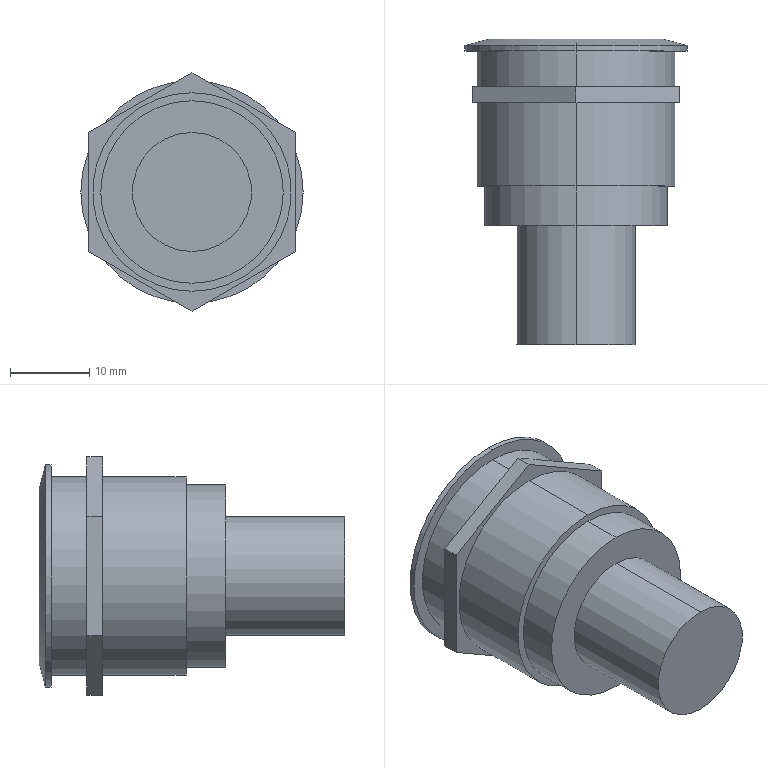Part | STEP file | MAIN_SWITCH_KNOB | 1 solid | 25 faces | box 28 x 38.5 x 30 mm | volume 14086 mm3 | plane 13 | cylinder 10 | cone 2 | commonest cylinder face diameters 25 x4 15 x2 23 x2 28 x2
STEP:
#1=CARTESIAN_POINT('',(0.,-8.,-12.5));
#2=VERTEX_POINT('',#1);
#3=CARTESIAN_POINT('',(0.,-8.,12.5));
#4=VERTEX_POINT('',#3);
#5=CARTESIAN_POINT('',(0.,-8.,0.));
#6=DIRECTION('',(0.,-1.,0.));
#7=DIRECTION('',(0.,0.,-1.));
#8=AXIS2_PLACEMENT_3D('',#5,#6,#7);
#9=CIRCLE('',#8,12.5);
#10=EDGE_CURVE('',#2,#4,#9,.T.);
#11=ORIENTED_EDGE('',*,*,#10,.T.);
#12=CARTESIAN_POINT('',(0.,-18.5,12.5));
#13=VERTEX_POINT('',#12);
#14=CARTESIAN_POINT('',(0.,1.925,12.5));
#15=DIRECTION('',(0.,-1.,0.));
#16=VECTOR('',#15,1000.);
#17=LINE('',#14,#16);
#18=EDGE_CURVE('',#4,#13,#17,.T.);
#19=ORIENTED_EDGE('',*,*,#18,.T.);
#20=CARTESIAN_POINT('',(0.,-18.5,-12.5));
#21=VERTEX_POINT('',#20);
#22=CARTESIAN_POINT('',(0.,-18.5,0.));
#23=DIRECTION('',(0.,1.,0.));
#24=DIRECTION('',(0.,0.,-1.));
#25=AXIS2_PLACEMENT_3D('',#22,#23,#24);
#26=CIRCLE('',#25,12.5);
#27=EDGE_CURVE('',#13,#21,#26,.T.);
#28=ORIENTED_EDGE('',*,*,#27,.T.);
#29=CARTESIAN_POINT('',(0.,1.925,-12.5));
#30=DIRECTION('',(0.,-1.,0.));
#31=VECTOR('',#30,1000.);
#32=LINE('',#29,#31);
#33=EDGE_CURVE('',#2,#21,#32,.T.);
#34=ORIENTED_EDGE('',*,*,#33,.F.);
#35=EDGE_LOOP('',(#11,#19,#28,#34));
#36=FACE_OUTER_BOUND('',#35,.T.);
#37=CARTESIAN_POINT('',(0.,1.925,0.));
#38=DIRECTION('',(0.,-1.,0.));
#39=DIRECTION('',(0.,0.,-1.));
#40=AXIS2_PLACEMENT_3D('',#37,#38,#39);
#41=CYLINDRICAL_SURFACE('',#40,12.5);
#42=ADVANCED_FACE('',(#36),#41,.T.);
#43=CARTESIAN_POINT('',(0.,-18.5,11.5));
#44=VERTEX_POINT('',#43);
#45=CARTESIAN_POINT('',(0.,-18.5,-11.5));
#46=VERTEX_POINT('',#45);
#47=CARTESIAN_POINT('',(0.,-18.5,0.));
#48=DIRECTION('',(0.,1.,0.));
#49=DIRECTION('',(0.,0.,-1.));
#50=AXIS2_PLACEMENT_3D('',#47,#48,#49);
#51=CIRCLE('',#50,11.5);
#52=EDGE_CURVE('',#44,#46,#51,.T.);
#53=ORIENTED_EDGE('',*,*,#52,.F.);
#54=CARTESIAN_POINT('',(0.,-23.5,11.5));
#55=VERTEX_POINT('',#54);
#56=CARTESIAN_POINT('',(0.,1.925,11.5));
#57=DIRECTION('',(0.,-1.,0.));
#58=VECTOR('',#57,1000.);
#59=LINE('',#56,#58);
#60=EDGE_CURVE('',#44,#55,#59,.T.);
#61=ORIENTED_EDGE('',*,*,#60,.T.);
#62=CARTESIAN_POINT('',(0.,-23.5,-11.5));
#63=VERTEX_POINT('',#62);
#64=CARTESIAN_POINT('',(0.,-23.5,0.));
#65=DIRECTION('',(0.,1.,0.));
#66=DIRECTION('',(0.,0.,-1.));
#67=AXIS2_PLACEMENT_3D('',#64,#65,#66);
#68=CIRCLE('',#67,11.5);
#69=EDGE_CURVE('',#55,#63,#68,.T.);
#70=ORIENTED_EDGE('',*,*,#69,.T.);
#71=CARTESIAN_POINT('',(0.,1.925,-11.5));
#72=DIRECTION('',(0.,-1.,0.));
#73=VECTOR('',#72,1000.);
#74=LINE('',#71,#73);
#75=EDGE_CURVE('',#46,#63,#74,.T.);
#76=ORIENTED_EDGE('',*,*,#75,.F.);
#77=EDGE_LOOP('',(#53,#61,#70,#76));
#78=FACE_OUTER_BOUND('',#77,.T.);
#79=CARTESIAN_POINT('',(0.,1.925,0.));
#80=DIRECTION('',(0.,-1.,0.));
#81=DIRECTION('',(0.,0.,-1.));
#82=AXIS2_PLACEMENT_3D('',#79,#80,#81);
#83=CYLINDRICAL_SURFACE('',#82,11.5);
#84=ADVANCED_FACE('',(#78),#83,.T.);
#85=CARTESIAN_POINT('',(0.,-23.5,7.5));
#86=VERTEX_POINT('',#85);
#87=CARTESIAN_POINT('',(0.,-23.5,-7.5));
#88=VERTEX_POINT('',#87);
#89=CARTESIAN_POINT('',(0.,-23.5,0.));
#90=DIRECTION('',(0.,1.,0.));
#91=DIRECTION('',(0.,0.,-1.));
#92=AXIS2_PLACEMENT_3D('',#89,#90,#91);
#93=CIRCLE('',#92,7.5);
#94=EDGE_CURVE('',#86,#88,#93,.T.);
#95=ORIENTED_EDGE('',*,*,#94,.F.);
#96=CARTESIAN_POINT('',(0.,-38.5,7.5));
#97=VERTEX_POINT('',#96);
#98=CARTESIAN_POINT('',(0.,1.925,7.5));
#99=DIRECTION('',(0.,-1.,0.));
#100=VECTOR('',#99,1000.);
#101=LINE('',#98,#100);
#102=EDGE_CURVE('',#86,#97,#101,.T.);
#103=ORIENTED_EDGE('',*,*,#102,.T.);
#104=CARTESIAN_POINT('',(0.,-38.5,-7.5));
#105=VERTEX_POINT('',#104);
#106=CARTESIAN_POINT('',(0.,-38.5,0.));
#107=DIRECTION('',(0.,1.,0.));
#108=DIRECTION('',(0.,0.,-1.));
#109=AXIS2_PLACEMENT_3D('',#106,#107,#108);
#110=CIRCLE('',#109,7.5);
#111=EDGE_CURVE('',#97,#105,#110,.T.);
#112=ORIENTED_EDGE('',*,*,#111,.T.);
#113=CARTESIAN_POINT('',(0.,1.925,-7.5));
#114=DIRECTION('',(0.,-1.,0.));
#115=VECTOR('',#114,1000.);
#116=LINE('',#113,#115);
#117=EDGE_CURVE('',#88,#105,#116,.T.);
#118=ORIENTED_EDGE('',*,*,#117,.F.);
#119=EDGE_LOOP('',(#95,#103,#112,#118));
#120=FACE_OUTER_BOUND('',#119,.T.);
#121=CARTESIAN_POINT('',(0.,1.925,0.));
#122=DIRECTION('',(0.,-1.,0.));
#123=DIRECTION('',(0.,0.,-1.));
#124=AXIS2_PLACEMENT_3D('',#121,#122,#123);
#125=CYLINDRICAL_SURFACE('',#124,7.5);
#126=ADVANCED_FACE('',(#120),#125,.T.);
#127=CARTESIAN_POINT('',(0.,-1.5,-12.5));
#128=VERTEX_POINT('',#127);
#129=CARTESIAN_POINT('',(0.,-1.5,12.5));
#130=VERTEX_POINT('',#129);
#131=CARTESIAN_POINT('',(0.,-1.5,0.));
#132=DIRECTION('',(0.,-1.,0.));
#133=DIRECTION('',(0.,0.,-1.));
#134=AXIS2_PLACEMENT_3D('',#131,#132,#133);
#135=CIRCLE('',#134,12.5);
#136=EDGE_CURVE('',#128,#130,#135,.T.);
#137=ORIENTED_EDGE('',*,*,#136,.T.);
#138=CARTESIAN_POINT('',(0.,-6.,12.5));
#139=VERTEX_POINT('',#138);
#140=CARTESIAN_POINT('',(0.,1.925,12.5));
#141=DIRECTION('',(0.,-1.,0.));
#142=VECTOR('',#141,1000.);
#143=LINE('',#140,#142);
#144=EDGE_CURVE('',#130,#139,#143,.T.);
#145=ORIENTED_EDGE('',*,*,#144,.T.);
#146=CARTESIAN_POINT('',(0.,-6.,-12.5));
#147=VERTEX_POINT('',#146);
#148=CARTESIAN_POINT('',(0.,-6.,0.));
#149=DIRECTION('',(0.,-1.,0.));
#150=DIRECTION('',(0.,0.,-1.));
#151=AXIS2_PLACEMENT_3D('',#148,#149,#150);
#152=CIRCLE('',#151,12.5);
#153=EDGE_CURVE('',#147,#139,#152,.T.);
#154=ORIENTED_EDGE('',*,*,#153,.F.);
#155=CARTESIAN_POINT('',(0.,1.925,-12.5));
#156=DIRECTION('',(0.,-1.,0.));
#157=VECTOR('',#156,1000.);
#158=LINE('',#155,#157);
#159=EDGE_CURVE('',#128,#147,#158,.T.);
#160=ORIENTED_EDGE('',*,*,#159,.F.);
#161=EDGE_LOOP('',(#137,#145,#154,#160));
#162=FACE_OUTER_BOUND('',#161,.T.);
#163=CARTESIAN_POINT('',(0.,1.925,0.));
#164=DIRECTION('',(0.,-1.,0.));
#165=DIRECTION('',(0.,0.,-1.));
#166=AXIS2_PLACEMENT_3D('',#163,#164,#165);
#167=CYLINDRICAL_SURFACE('',#166,12.5);
#168=ADVANCED_FACE('',(#162),#167,.T.);
#169=CARTESIAN_POINT('',(0.,-0.8,-14.));
#170=VERTEX_POINT('',#169);
#171=CARTESIAN_POINT('',(0.,-0.8,14.));
#172=VERTEX_POINT('',#171);
#173=CARTESIAN_POINT('',(0.,-0.8,0.));
#174=DIRECTION('',(0.,-1.,0.));
#175=DIRECTION('',(0.,0.,-1.));
#176=AXIS2_PLACEMENT_3D('',#173,#174,#175);
#177=CIRCLE('',#176,14.);
#178=EDGE_CURVE('',#170,#172,#177,.T.);
#179=ORIENTED_EDGE('',*,*,#178,.T.);
#180=CARTESIAN_POINT('',(0.,-1.5,14.));
#181=VERTEX_POINT('',#180);
#182=CARTESIAN_POINT('',(0.,1.925,14.));
#183=DIRECTION('',(0.,-1.,0.));
#184=VECTOR('',#183,1000.);
#185=LINE('',#182,#184);
#186=EDGE_CURVE('',#172,#181,#185,.T.);
#187=ORIENTED_EDGE('',*,*,#186,.T.);
#188=CARTESIAN_POINT('',(0.,-1.5,-14.));
#189=VERTEX_POINT('',#188);
#190=CARTESIAN_POINT('',(0.,-1.5,0.));
#191=DIRECTION('',(0.,-1.,0.));
#192=DIRECTION('',(0.,0.,-1.));
#193=AXIS2_PLACEMENT_3D('',#190,#191,#192);
#194=CIRCLE('',#193,14.);
#195=EDGE_CURVE('',#189,#181,#194,.T.);
#196=ORIENTED_EDGE('',*,*,#195,.F.);
#197=CARTESIAN_POINT('',(0.,1.925,-14.));
#198=DIRECTION('',(0.,-1.,0.));
#199=VECTOR('',#198,1000.);
#200=LINE('',#197,#199);
#201=EDGE_CURVE('',#170,#189,#200,.T.);
#202=ORIENTED_EDGE('',*,*,#201,.F.);
#203=EDGE_LOOP('',(#179,#187,#196,#202));
#204=FACE_OUTER_BOUND('',#203,.T.);
#205=CARTESIAN_POINT('',(0.,1.925,0.));
#206=DIRECTION('',(0.,-1.,0.));
#207=DIRECTION('',(0.,0.,-1.));
#208=AXIS2_PLACEMENT_3D('',#205,#206,#207);
#209=CYLINDRICAL_SURFACE('',#208,14.);
#210=ADVANCED_FACE('',(#204),#209,.T.);
#211=CARTESIAN_POINT('',(0.,0.,-11.014));
#212=VERTEX_POINT('',#211);
#213=CARTESIAN_POINT('',(0.,0.,11.014));
#214=VERTEX_POINT('',#213);
#215=CARTESIAN_POINT('',(0.,0.,0.));
#216=DIRECTION('',(0.,-1.,0.));
#217=DIRECTION('',(0.,0.,-1.));
#218=AXIS2_PLACEMENT_3D('',#215,#216,#217);
#219=CIRCLE('',#218,11.014);
#220=EDGE_CURVE('',#212,#214,#219,.T.);
#221=ORIENTED_EDGE('',*,*,#220,.T.);
#222=CARTESIAN_POINT('',(0.,-0.8,14.));
#223=DIRECTION('',(0.,-0.2588,0.9659));
#224=VECTOR('',#223,1000.);
#225=LINE('',#222,#224);
#226=EDGE_CURVE('',#214,#172,#225,.T.);
#227=ORIENTED_EDGE('',*,*,#226,.T.);
#228=ORIENTED_EDGE('',*,*,#178,.F.);
#229=CARTESIAN_POINT('',(0.,-0.8,-14.));
#230=DIRECTION('',(0.,-0.2588,-0.9659));
#231=VECTOR('',#230,1000.);
#232=LINE('',#229,#231);
#233=EDGE_CURVE('',#212,#170,#232,.T.);
#234=ORIENTED_EDGE('',*,*,#233,.F.);
#235=EDGE_LOOP('',(#221,#227,#228,#234));
#236=FACE_OUTER_BOUND('',#235,.T.);
#237=CARTESIAN_POINT('',(0.,-0.8,0.));
#238=DIRECTION('',(0.,-1.,0.));
#239=DIRECTION('',(0.,0.,-1.));
#240=AXIS2_PLACEMENT_3D('',#237,#238,#239);
#241=CONICAL_SURFACE('',#240,14.,1.309);
#242=ADVANCED_FACE('',(#236),#241,.T.);
#243=ORIENTED_EDGE('',*,*,#18,.F.);
#244=CARTESIAN_POINT('',(0.,-8.,0.));
#245=DIRECTION('',(0.,-1.,0.));
#246=DIRECTION('',(0.,0.,-1.));
#247=AXIS2_PLACEMENT_3D('',#244,#245,#246);
#248=CIRCLE('',#247,12.5);
#249=EDGE_CURVE('',#4,#2,#248,.T.);
#250=ORIENTED_EDGE('',*,*,#249,.T.);
#251=ORIENTED_EDGE('',*,*,#33,.T.);
#252=CARTESIAN_POINT('',(0.,-18.5,0.));
#253=DIRECTION('',(0.,1.,0.));
#254=DIRECTION('',(0.,0.,-1.));
#255=AXIS2_PLACEMENT_3D('',#252,#253,#254);
#256=CIRCLE('',#255,12.5);
#257=EDGE_CURVE('',#21,#13,#256,.T.);
#258=ORIENTED_EDGE('',*,*,#257,.T.);
#259=EDGE_LOOP('',(#243,#250,#251,#258));
#260=FACE_OUTER_BOUND('',#259,.T.);
#261=CARTESIAN_POINT('',(0.,1.925,0.));
#262=DIRECTION('',(0.,-1.,0.));
#263=DIRECTION('',(0.,0.,-1.));
#264=AXIS2_PLACEMENT_3D('',#261,#262,#263);
#265=CYLINDRICAL_SURFACE('',#264,12.5);
#266=ADVANCED_FACE('',(#260),#265,.T.);
#267=CARTESIAN_POINT('',(0.,-18.5,0.));
#268=DIRECTION('',(0.,1.,0.));
#269=DIRECTION('',(0.,0.,-1.));
#270=AXIS2_PLACEMENT_3D('',#267,#268,#269);
#271=CIRCLE('',#270,11.5);
#272=EDGE_CURVE('',#46,#44,#271,.T.);
#273=ORIENTED_EDGE('',*,*,#272,.T.);
#274=ORIENTED_EDGE('',*,*,#52,.T.);
#275=EDGE_LOOP('',(#273,#274));
#276=FACE_BOUND('',#275,.T.);
#277=ORIENTED_EDGE('',*,*,#257,.F.);
#278=ORIENTED_EDGE('',*,*,#27,.F.);
#279=EDGE_LOOP('',(#277,#278));
#280=FACE_OUTER_BOUND('',#279,.T.);
#281=CARTESIAN_POINT('',(0.,-18.5,0.));
#282=DIRECTION('',(0.,-1.,0.));
#283=DIRECTION('',(0.,0.,-1.));
#284=AXIS2_PLACEMENT_3D('',#281,#282,#283);
#285=PLANE('',#284);
#286=ADVANCED_FACE('',(#276,#280),#285,.T.);
#287=ORIENTED_EDGE('',*,*,#10,.F.);
#288=ORIENTED_EDGE('',*,*,#249,.F.);
#289=EDGE_LOOP('',(#287,#288));
#290=FACE_BOUND('',#289,.T.);
#291=CARTESIAN_POINT('',(0.,-8.,-15.));
#292=VERTEX_POINT('',#291);
#293=CARTESIAN_POINT('',(-12.99,-8.,-7.5));
#294=VERTEX_POINT('',#293);
#295=CARTESIAN_POINT('',(0.,-8.,-15.));
#296=DIRECTION('',(-0.866,0.,0.5));
#297=VECTOR('',#296,1000.);
#298=LINE('',#295,#297);
#299=EDGE_CURVE('',#292,#294,#298,.T.);
#300=ORIENTED_EDGE('',*,*,#299,.F.);
#301=CARTESIAN_POINT('',(12.99,-8.,-7.5));
#302=VERTEX_POINT('',#301);
#303=CARTESIAN_POINT('',(12.99,-8.,-7.5));
#304=DIRECTION('',(-0.866,0.,-0.5));
#305=VECTOR('',#304,1000.);
#306=LINE('',#303,#305);
#307=EDGE_CURVE('',#302,#292,#306,.T.);
#308=ORIENTED_EDGE('',*,*,#307,.F.);
#309=CARTESIAN_POINT('',(12.99,-8.,7.5));
#310=VERTEX_POINT('',#309);
#311=CARTESIAN_POINT('',(12.99,-8.,0.));
#312=DIRECTION('',(0.,0.,-1.));
#313=VECTOR('',#312,1000.);
#314=LINE('',#311,#313);
#315=EDGE_CURVE('',#310,#302,#314,.T.);
#316=ORIENTED_EDGE('',*,*,#315,.F.);
#317=CARTESIAN_POINT('',(0.,-8.,15.));
#318=VERTEX_POINT('',#317);
#319=CARTESIAN_POINT('',(0.,-8.,15.));
#320=DIRECTION('',(0.866,0.,-0.5));
#321=VECTOR('',#320,1000.);
#322=LINE('',#319,#321);
#323=EDGE_CURVE('',#318,#310,#322,.T.);
#324=ORIENTED_EDGE('',*,*,#323,.F.);
#325=CARTESIAN_POINT('',(-12.99,-8.,7.5));
#326=VERTEX_POINT('',#325);
#327=CARTESIAN_POINT('',(-12.99,-8.,7.5));
#328=DIRECTION('',(0.866,0.,0.5));
#329=VECTOR('',#328,1000.);
#330=LINE('',#327,#329);
#331=EDGE_CURVE('',#326,#318,#330,.T.);
#332=ORIENTED_EDGE('',*,*,#331,.F.);
#333=CARTESIAN_POINT('',(-12.99,-8.,0.));
#334=DIRECTION('',(0.,0.,1.));
#335=VECTOR('',#334,1000.);
#336=LINE('',#333,#335);
#337=EDGE_CURVE('',#294,#326,#336,.T.);
#338=ORIENTED_EDGE('',*,*,#337,.F.);
#339=EDGE_LOOP('',(#300,#308,#316,#324,#332,#338));
#340=FACE_OUTER_BOUND('',#339,.T.);
#341=CARTESIAN_POINT('',(0.,-8.,0.));
#342=DIRECTION('',(0.,1.,0.));
#343=DIRECTION('',(0.,0.,1.));
#344=AXIS2_PLACEMENT_3D('',#341,#342,#343);
#345=PLANE('',#344);
#346=ADVANCED_FACE('',(#290,#340),#345,.F.);
#347=ORIENTED_EDGE('',*,*,#60,.F.);
#348=ORIENTED_EDGE('',*,*,#272,.F.);
#349=ORIENTED_EDGE('',*,*,#75,.T.);
#350=CARTESIAN_POINT('',(0.,-23.5,0.));
#351=DIRECTION('',(0.,1.,0.));
#352=DIRECTION('',(0.,0.,-1.));
#353=AXIS2_PLACEMENT_3D('',#350,#351,#352);
#354=CIRCLE('',#353,11.5);
#355=EDGE_CURVE('',#63,#55,#354,.T.);
#356=ORIENTED_EDGE('',*,*,#355,.T.);
#357=EDGE_LOOP('',(#347,#348,#349,#356));
#358=FACE_OUTER_BOUND('',#357,.T.);
#359=CARTESIAN_POINT('',(0.,1.925,0.));
#360=DIRECTION('',(0.,-1.,0.));
#361=DIRECTION('',(0.,0.,-1.));
#362=AXIS2_PLACEMENT_3D('',#359,#360,#361);
#363=CYLINDRICAL_SURFACE('',#362,11.5);
#364=ADVANCED_FACE('',(#358),#363,.T.);
#365=CARTESIAN_POINT('',(-12.99,-6.,-7.5));
#366=VERTEX_POINT('',#365);
#367=CARTESIAN_POINT('',(-12.99,-8.,-7.5));
#368=DIRECTION('',(0.,-1.,0.));
#369=VECTOR('',#368,1000.);
#370=LINE('',#367,#369);
#371=EDGE_CURVE('',#366,#294,#370,.T.);
#372=ORIENTED_EDGE('',*,*,#371,.T.);
#373=ORIENTED_EDGE('',*,*,#337,.T.);
#374=CARTESIAN_POINT('',(-12.99,-6.,7.5));
#375=VERTEX_POINT('',#374);
#376=CARTESIAN_POINT('',(-12.99,-8.,7.5));
#377=DIRECTION('',(0.,1.,0.));
#378=VECTOR('',#377,1000.);
#379=LINE('',#376,#378);
#380=EDGE_CURVE('',#326,#375,#379,.T.);
#381=ORIENTED_EDGE('',*,*,#380,.T.);
#382=CARTESIAN_POINT('',(-12.99,-6.,-7.5));
#383=DIRECTION('',(0.,0.,-1.));
#384=VECTOR('',#383,1000.);
#385=LINE('',#382,#384);
#386=EDGE_CURVE('',#375,#366,#385,.T.);
#387=ORIENTED_EDGE('',*,*,#386,.T.);
#388=EDGE_LOOP('',(#372,#373,#381,#387));
#389=FACE_OUTER_BOUND('',#388,.T.);
#390=CARTESIAN_POINT('',(-12.99,-8.,-7.5));
#391=DIRECTION('',(-1.,0.,0.));
#392=DIRECTION('',(0.,0.,1.));
#393=AXIS2_PLACEMENT_3D('',#390,#391,#392);
#394=PLANE('',#393);
#395=ADVANCED_FACE('',(#389),#394,.T.);
#396=CARTESIAN_POINT('',(0.,-6.,-15.));
#397=VERTEX_POINT('',#396);
#398=CARTESIAN_POINT('',(0.,-8.,-15.));
#399=DIRECTION('',(0.,-1.,0.));
#400=VECTOR('',#399,1000.);
#401=LINE('',#398,#400);
#402=EDGE_CURVE('',#397,#292,#401,.T.);
#403=ORIENTED_EDGE('',*,*,#402,.T.);
#404=ORIENTED_EDGE('',*,*,#299,.T.);
#405=ORIENTED_EDGE('',*,*,#371,.F.);
#406=CARTESIAN_POINT('',(0.,-6.,-15.));
#407=DIRECTION('',(0.866,0.,-0.5));
#408=VECTOR('',#407,1000.);
#409=LINE('',#406,#408);
#410=EDGE_CURVE('',#366,#397,#409,.T.);
#411=ORIENTED_EDGE('',*,*,#410,.T.);
#412=EDGE_LOOP('',(#403,#404,#405,#411));
#413=FACE_OUTER_BOUND('',#412,.T.);
#414=CARTESIAN_POINT('',(0.,-8.,-15.));
#415=DIRECTION('',(-0.5,0.,-0.866));
#416=DIRECTION('',(-0.866,0.,0.5));
#417=AXIS2_PLACEMENT_3D('',#414,#415,#416);
#418=PLANE('',#417);
#419=ADVANCED_FACE('',(#413),#418,.T.);
#420=CARTESIAN_POINT('',(12.99,-6.,-7.5));
#421=VERTEX_POINT('',#420);
#422=CARTESIAN_POINT('',(12.99,-8.,-7.5));
#423=DIRECTION('',(0.,-1.,0.));
#424=VECTOR('',#423,1000.);
#425=LINE('',#422,#424);
#426=EDGE_CURVE('',#421,#302,#425,.T.);
#427=ORIENTED_EDGE('',*,*,#426,.T.);
#428=ORIENTED_EDGE('',*,*,#307,.T.);
#429=ORIENTED_EDGE('',*,*,#402,.F.);
#430=CARTESIAN_POINT('',(12.99,-6.,-7.5));
#431=DIRECTION('',(0.866,0.,0.5));
#432=VECTOR('',#431,1000.);
#433=LINE('',#430,#432);
#434=EDGE_CURVE('',#397,#421,#433,.T.);
#435=ORIENTED_EDGE('',*,*,#434,.T.);
#436=EDGE_LOOP('',(#427,#428,#429,#435));
#437=FACE_OUTER_BOUND('',#436,.T.);
#438=CARTESIAN_POINT('',(12.99,-8.,-7.5));
#439=DIRECTION('',(0.5,0.,-0.866));
#440=DIRECTION('',(-0.866,0.,-0.5));
#441=AXIS2_PLACEMENT_3D('',#438,#439,#440);
#442=PLANE('',#441);
#443=ADVANCED_FACE('',(#437),#442,.T.);
#444=CARTESIAN_POINT('',(12.99,-6.,7.5));
#445=VERTEX_POINT('',#444);
#446=CARTESIAN_POINT('',(12.99,-8.,7.5));
#447=DIRECTION('',(0.,-1.,0.));
#448=VECTOR('',#447,1000.);
#449=LINE('',#446,#448);
#450=EDGE_CURVE('',#445,#310,#449,.T.);
#451=ORIENTED_EDGE('',*,*,#450,.T.);
#452=ORIENTED_EDGE('',*,*,#315,.T.);
#453=ORIENTED_EDGE('',*,*,#426,.F.);
#454=CARTESIAN_POINT('',(12.99,-6.,7.5));
#455=DIRECTION('',(0.,0.,1.));
#456=VECTOR('',#455,1000.);
#457=LINE('',#454,#456);
#458=EDGE_CURVE('',#421,#445,#457,.T.);
#459=ORIENTED_EDGE('',*,*,#458,.T.);
#460=EDGE_LOOP('',(#451,#452,#453,#459));
#461=FACE_OUTER_BOUND('',#460,.T.);
#462=CARTESIAN_POINT('',(12.99,-8.,7.5));
#463=DIRECTION('',(1.,0.,0.));
#464=DIRECTION('',(0.,0.,-1.));
#465=AXIS2_PLACEMENT_3D('',#462,#463,#464);
#466=PLANE('',#465);
#467=ADVANCED_FACE('',(#461),#466,.T.);
#468=CARTESIAN_POINT('',(0.,-6.,15.));
#469=VERTEX_POINT('',#468);
#470=CARTESIAN_POINT('',(0.,-8.,15.));
#471=DIRECTION('',(0.,-1.,0.));
#472=VECTOR('',#471,1000.);
#473=LINE('',#470,#472);
#474=EDGE_CURVE('',#469,#318,#473,.T.);
#475=ORIENTED_EDGE('',*,*,#474,.T.);
#476=ORIENTED_EDGE('',*,*,#323,.T.);
#477=ORIENTED_EDGE('',*,*,#450,.F.);
#478=CARTESIAN_POINT('',(0.,-6.,15.));
#479=DIRECTION('',(-0.866,0.,0.5));
#480=VECTOR('',#479,1000.);
#481=LINE('',#478,#480);
#482=EDGE_CURVE('',#445,#469,#481,.T.);
#483=ORIENTED_EDGE('',*,*,#482,.T.);
#484=EDGE_LOOP('',(#475,#476,#477,#483));
#485=FACE_OUTER_BOUND('',#484,.T.);
#486=CARTESIAN_POINT('',(0.,-8.,15.));
#487=DIRECTION('',(0.5,0.,0.866));
#488=DIRECTION('',(0.866,0.,-0.5));
#489=AXIS2_PLACEMENT_3D('',#486,#487,#488);
#490=PLANE('',#489);
#491=ADVANCED_FACE('',(#485),#490,.T.);
#492=ORIENTED_EDGE('',*,*,#380,.F.);
#493=ORIENTED_EDGE('',*,*,#331,.T.);
#494=ORIENTED_EDGE('',*,*,#474,.F.);
#495=CARTESIAN_POINT('',(-12.99,-6.,7.5));
#496=DIRECTION('',(-0.866,0.,-0.5));
#497=VECTOR('',#496,1000.);
#498=LINE('',#495,#497);
#499=EDGE_CURVE('',#469,#375,#498,.T.);
#500=ORIENTED_EDGE('',*,*,#499,.T.);
#501=EDGE_LOOP('',(#492,#493,#494,#500));
#502=FACE_OUTER_BOUND('',#501,.T.);
#503=CARTESIAN_POINT('',(-12.99,-8.,7.5));
#504=DIRECTION('',(-0.5,0.,0.866));
#505=DIRECTION('',(0.866,0.,0.5));
#506=AXIS2_PLACEMENT_3D('',#503,#504,#505);
#507=PLANE('',#506);
#508=ADVANCED_FACE('',(#502),#507,.T.);
#509=CARTESIAN_POINT('',(0.,-23.5,0.));
#510=DIRECTION('',(0.,1.,0.));
#511=DIRECTION('',(0.,0.,-1.));
#512=AXIS2_PLACEMENT_3D('',#509,#510,#511);
#513=CIRCLE('',#512,7.5);
#514=EDGE_CURVE('',#88,#86,#513,.T.);
#515=ORIENTED_EDGE('',*,*,#514,.T.);
#516=ORIENTED_EDGE('',*,*,#94,.T.);
#517=EDGE_LOOP('',(#515,#516));
#518=FACE_BOUND('',#517,.T.);
#519=ORIENTED_EDGE('',*,*,#355,.F.);
#520=ORIENTED_EDGE('',*,*,#69,.F.);
#521=EDGE_LOOP('',(#519,#520));
#522=FACE_OUTER_BOUND('',#521,.T.);
#523=CARTESIAN_POINT('',(0.,-23.5,0.));
#524=DIRECTION('',(0.,-1.,0.));
#525=DIRECTION('',(0.,0.,-1.));
#526=AXIS2_PLACEMENT_3D('',#523,#524,#525);
#527=PLANE('',#526);
#528=ADVANCED_FACE('',(#518,#522),#527,.T.);
#529=ORIENTED_EDGE('',*,*,#153,.T.);
#530=CARTESIAN_POINT('',(0.,-6.,0.));
#531=DIRECTION('',(0.,-1.,0.));
#532=DIRECTION('',(0.,0.,-1.));
#533=AXIS2_PLACEMENT_3D('',#530,#531,#532);
#534=CIRCLE('',#533,12.5);
#535=EDGE_CURVE('',#139,#147,#534,.T.);
#536=ORIENTED_EDGE('',*,*,#535,.T.);
#537=EDGE_LOOP('',(#529,#536));
#538=FACE_BOUND('',#537,.T.);
#539=ORIENTED_EDGE('',*,*,#434,.F.);
#540=ORIENTED_EDGE('',*,*,#410,.F.);
#541=ORIENTED_EDGE('',*,*,#386,.F.);
#542=ORIENTED_EDGE('',*,*,#499,.F.);
#543=ORIENTED_EDGE('',*,*,#482,.F.);
#544=ORIENTED_EDGE('',*,*,#458,.F.);
#545=EDGE_LOOP('',(#539,#540,#541,#542,#543,#544));
#546=FACE_OUTER_BOUND('',#545,.T.);
#547=CARTESIAN_POINT('',(0.,-6.,0.));
#548=DIRECTION('',(0.,1.,0.));
#549=DIRECTION('',(0.,0.,1.));
#550=AXIS2_PLACEMENT_3D('',#547,#548,#549);
#551=PLANE('',#550);
#552=ADVANCED_FACE('',(#538,#546),#551,.T.);
#553=ORIENTED_EDGE('',*,*,#102,.F.);
#554=ORIENTED_EDGE('',*,*,#514,.F.);
#555=ORIENTED_EDGE('',*,*,#117,.T.);
#556=CARTESIAN_POINT('',(0.,-38.5,0.));
#557=DIRECTION('',(0.,1.,0.));
#558=DIRECTION('',(0.,0.,-1.));
#559=AXIS2_PLACEMENT_3D('',#556,#557,#558);
#560=CIRCLE('',#559,7.5);
#561=EDGE_CURVE('',#105,#97,#560,.T.);
#562=ORIENTED_EDGE('',*,*,#561,.T.);
#563=EDGE_LOOP('',(#553,#554,#555,#562));
#564=FACE_OUTER_BOUND('',#563,.T.);
#565=CARTESIAN_POINT('',(0.,1.925,0.));
#566=DIRECTION('',(0.,-1.,0.));
#567=DIRECTION('',(0.,0.,-1.));
#568=AXIS2_PLACEMENT_3D('',#565,#566,#567);
#569=CYLINDRICAL_SURFACE('',#568,7.5);
#570=ADVANCED_FACE('',(#564),#569,.T.);
#571=ORIENTED_EDGE('',*,*,#144,.F.);
#572=CARTESIAN_POINT('',(0.,-1.5,0.));
#573=DIRECTION('',(0.,-1.,0.));
#574=DIRECTION('',(0.,0.,-1.));
#575=AXIS2_PLACEMENT_3D('',#572,#573,#574);
#576=CIRCLE('',#575,12.5);
#577=EDGE_CURVE('',#130,#128,#576,.T.);
#578=ORIENTED_EDGE('',*,*,#577,.T.);
#579=ORIENTED_EDGE('',*,*,#159,.T.);
#580=ORIENTED_EDGE('',*,*,#535,.F.);
#581=EDGE_LOOP('',(#571,#578,#579,#580));
#582=FACE_OUTER_BOUND('',#581,.T.);
#583=CARTESIAN_POINT('',(0.,1.925,0.));
#584=DIRECTION('',(0.,-1.,0.));
#585=DIRECTION('',(0.,0.,-1.));
#586=AXIS2_PLACEMENT_3D('',#583,#584,#585);
#587=CYLINDRICAL_SURFACE('',#586,12.5);
#588=ADVANCED_FACE('',(#582),#587,.T.);
#589=ORIENTED_EDGE('',*,*,#561,.F.);
#590=ORIENTED_EDGE('',*,*,#111,.F.);
#591=EDGE_LOOP('',(#589,#590));
#592=FACE_OUTER_BOUND('',#591,.T.);
#593=CARTESIAN_POINT('',(0.,-38.5,0.));
#594=DIRECTION('',(0.,-1.,0.));
#595=DIRECTION('',(0.,0.,-1.));
#596=AXIS2_PLACEMENT_3D('',#593,#594,#595);
#597=PLANE('',#596);
#598=ADVANCED_FACE('',(#592),#597,.T.);
#599=ORIENTED_EDGE('',*,*,#136,.F.);
#600=ORIENTED_EDGE('',*,*,#577,.F.);
#601=EDGE_LOOP('',(#599,#600));
#602=FACE_BOUND('',#601,.T.);
#603=ORIENTED_EDGE('',*,*,#195,.T.);
#604=CARTESIAN_POINT('',(0.,-1.5,0.));
#605=DIRECTION('',(0.,-1.,0.));
#606=DIRECTION('',(0.,0.,-1.));
#607=AXIS2_PLACEMENT_3D('',#604,#605,#606);
#608=CIRCLE('',#607,14.);
#609=EDGE_CURVE('',#181,#189,#608,.T.);
#610=ORIENTED_EDGE('',*,*,#609,.T.);
#611=EDGE_LOOP('',(#603,#610));
#612=FACE_OUTER_BOUND('',#611,.T.);
#613=CARTESIAN_POINT('',(0.,-1.5,0.));
#614=DIRECTION('',(0.,-1.,0.));
#615=DIRECTION('',(0.,0.,-1.));
#616=AXIS2_PLACEMENT_3D('',#613,#614,#615);
#617=PLANE('',#616);
#618=ADVANCED_FACE('',(#602,#612),#617,.T.);
#619=ORIENTED_EDGE('',*,*,#186,.F.);
#620=CARTESIAN_POINT('',(0.,-0.8,0.));
#621=DIRECTION('',(0.,-1.,0.));
#622=DIRECTION('',(0.,0.,-1.));
#623=AXIS2_PLACEMENT_3D('',#620,#621,#622);
#624=CIRCLE('',#623,14.);
#625=EDGE_CURVE('',#172,#170,#624,.T.);
#626=ORIENTED_EDGE('',*,*,#625,.T.);
#627=ORIENTED_EDGE('',*,*,#201,.T.);
#628=ORIENTED_EDGE('',*,*,#609,.F.);
#629=EDGE_LOOP('',(#619,#626,#627,#628));
#630=FACE_OUTER_BOUND('',#629,.T.);
#631=CARTESIAN_POINT('',(0.,1.925,0.));
#632=DIRECTION('',(0.,-1.,0.));
#633=DIRECTION('',(0.,0.,-1.));
#634=AXIS2_PLACEMENT_3D('',#631,#632,#633);
#635=CYLINDRICAL_SURFACE('',#634,14.);
#636=ADVANCED_FACE('',(#630),#635,.T.);
#637=ORIENTED_EDGE('',*,*,#226,.F.);
#638=CARTESIAN_POINT('',(0.,0.,0.));
#639=DIRECTION('',(0.,-1.,0.));
#640=DIRECTION('',(0.,0.,-1.));
#641=AXIS2_PLACEMENT_3D('',#638,#639,#640);
#642=CIRCLE('',#641,11.014);
#643=EDGE_CURVE('',#214,#212,#642,.T.);
#644=ORIENTED_EDGE('',*,*,#643,.T.);
#645=ORIENTED_EDGE('',*,*,#233,.T.);
#646=ORIENTED_EDGE('',*,*,#625,.F.);
#647=EDGE_LOOP('',(#637,#644,#645,#646));
#648=FACE_OUTER_BOUND('',#647,.T.);
#649=CARTESIAN_POINT('',(0.,-0.8,0.));
#650=DIRECTION('',(0.,-1.,0.));
#651=DIRECTION('',(0.,0.,-1.));
#652=AXIS2_PLACEMENT_3D('',#649,#650,#651);
#653=CONICAL_SURFACE('',#652,14.,1.309);
#654=ADVANCED_FACE('',(#648),#653,.T.);
#655=ORIENTED_EDGE('',*,*,#220,.F.);
#656=ORIENTED_EDGE('',*,*,#643,.F.);
#657=EDGE_LOOP('',(#655,#656));
#658=FACE_OUTER_BOUND('',#657,.T.);
#659=CARTESIAN_POINT('',(0.,0.,0.));
#660=DIRECTION('',(0.,-1.,0.));
#661=DIRECTION('',(0.,0.,-1.));
#662=AXIS2_PLACEMENT_3D('',#659,#660,#661);
#663=PLANE('',#662);
#664=ADVANCED_FACE('',(#658),#663,.F.);
#665=CLOSED_SHELL('',(#42,#84,#126,#168,#210,#242,#266,#286,#346,#364,#395,#419,#443,#467,#491,#508,#528,#552,#570,#588,#598,#618,#636,#654,#664));
#666=MANIFOLD_SOLID_BREP('',#665);
#667=CARTESIAN_POINT('',(0.,0.,0.));
#668=DIRECTION('',(0.,0.,1.));
#669=DIRECTION('',(1.,0.,0.));
#670=AXIS2_PLACEMENT_3D('',#667,#668,#669);
#671=(LENGTH_UNIT()NAMED_UNIT(*)SI_UNIT(.MILLI.,.METRE.));
#672=UNCERTAINTY_MEASURE_WITH_UNIT(LENGTH_MEASURE(0.00001),#671,'','');
#673=(NAMED_UNIT(*)PLANE_ANGLE_UNIT()SI_UNIT($,.RADIAN.));
#674=(NAMED_UNIT(*)SI_UNIT($,.STERADIAN.)SOLID_ANGLE_UNIT());
#675=(GEOMETRIC_REPRESENTATION_CONTEXT(3)GLOBAL_UNCERTAINTY_ASSIGNED_CONTEXT((#672))GLOBAL_UNIT_ASSIGNED_CONTEXT((#671,#673,#674))REPRESENTATION_CONTEXT('',''));
#676=ADVANCED_BREP_SHAPE_REPRESENTATION('',(#666,#670),#675);